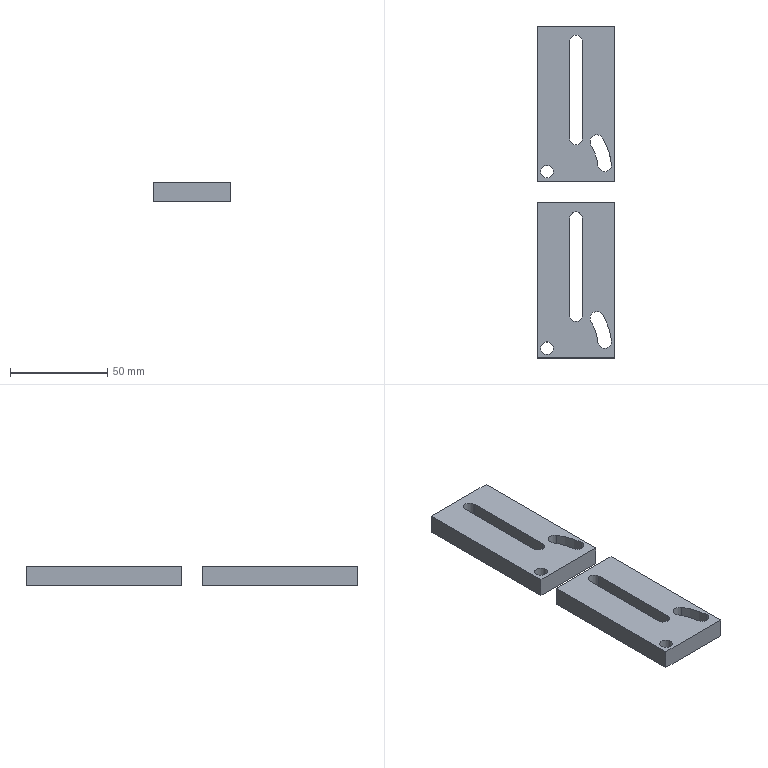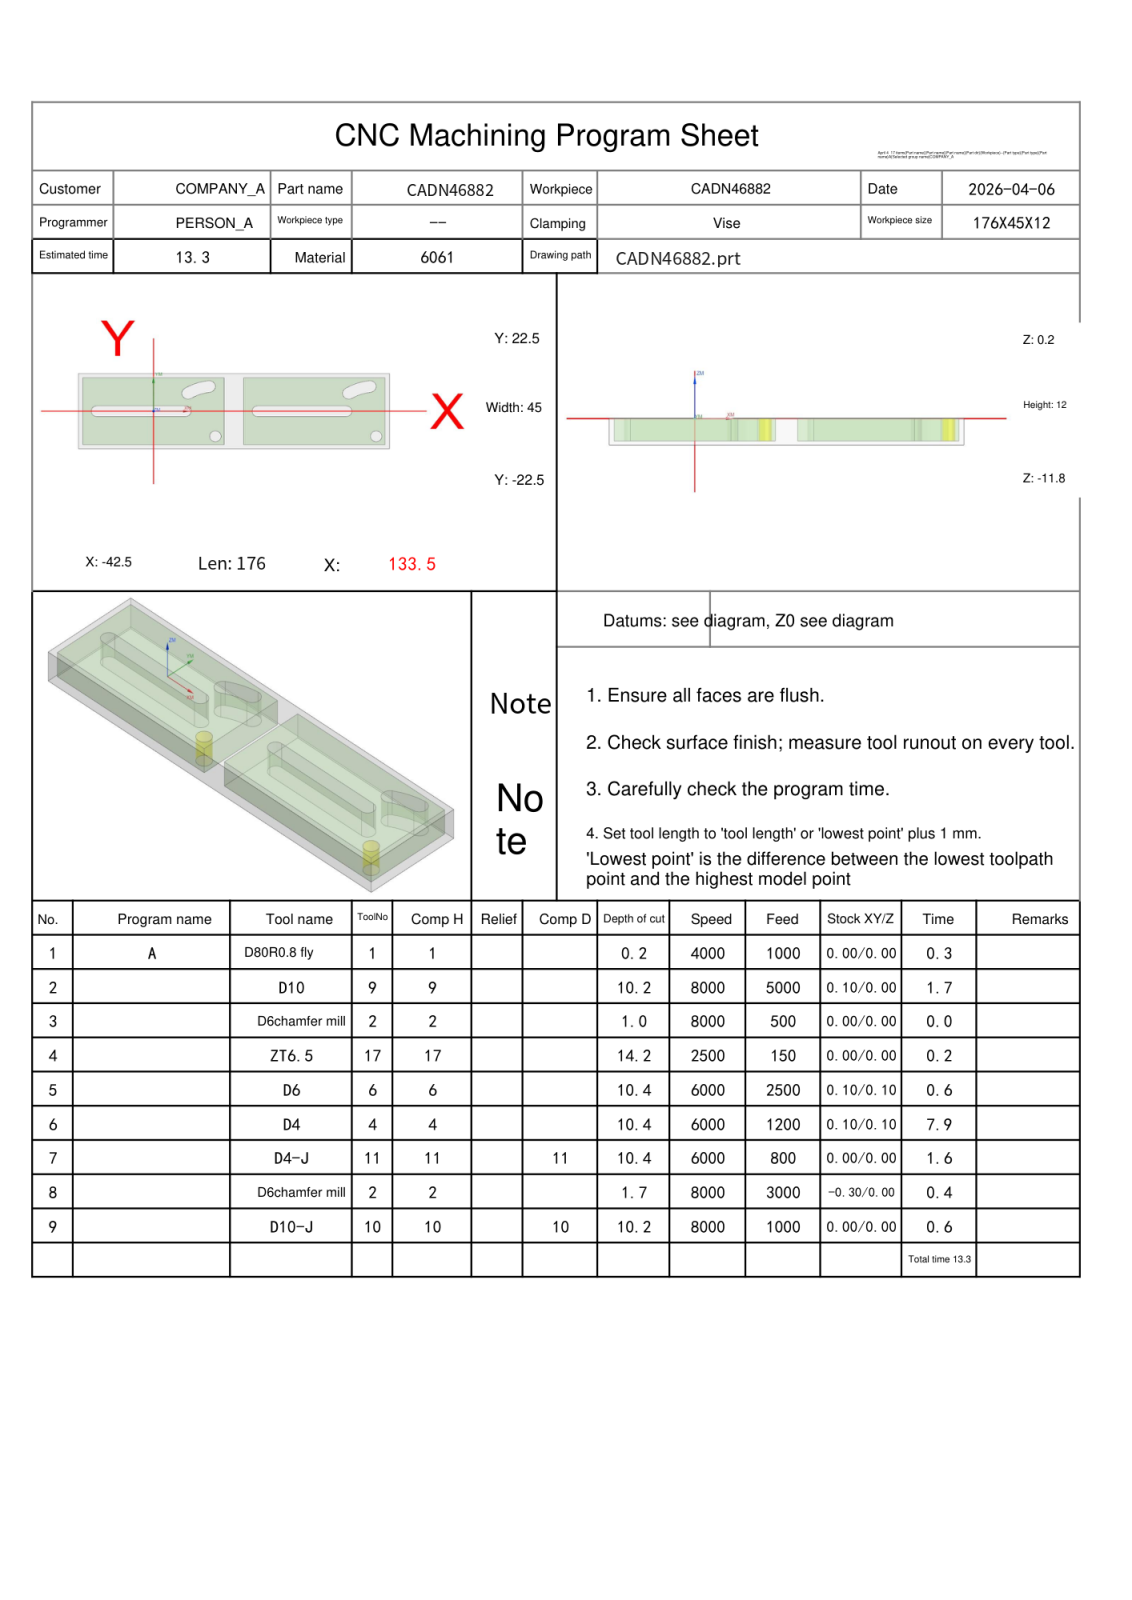NC program | NX | posted by the shop | part box 40 x 171 x 10 mm
Lines 1 to 1759 of 1806, first 1216 of 1757 lines:
%
O0001
(Machine time: 15.00 MIN)
(===Total Tool:8===)
(T1=D80R0.8 fly D=80.  R=0.8  D-  H01 Z=0.    )
(T9=D10     D=10.  R=0.   D-  H09 Z=-10.  )
(T2=D6chamfer mill   D=6.   R=0.   D-  H02 Z=-1.5  )
(T17=ZT6.5  D=6.5  DR_a=118 D-  H17 Z=-13.95)
(T6=D6      D=6.   R=0.   D-  H06 Z=-10.2 )
(T4=D4      D=4.   R=0.   D-  H04 Z=-10.2 )
(T11=D4-J   D=4.   R=0.   D11 H11 Z=-10.2 )
(T10=D10-J  D=10.  R=0.   D10 H10 Z=-10.  )
G80 G90 G17 G49 G40
G91 G28 Z0
M01
N1 T01 M06
(D80R0.8 fly  D=80. R=0.8 H=01 ce=0.00 di=0.00)
G00 G90 G54 X176. Y0.0 M03 S4000
G43 H01 Z20.
M08
Z2.
G01 Z0.0 F1000.
X171.
X-80.
X-85.
Z2.
G00 Z20.
G91 G28 Z0.0
M05
M09
G91 G28 Z0.0
M01
N2 T09 M06
(D10  D=10. R=0. H=09 ce=0.10 di=0.00)
G00 G90 G54 X91. Y-25.1 M03 S8000
G43 H09 Z20.
M08
Z.5
G01 X51. Z.39 F5000.
G02 X45.9 Y-20. Z.368 I0.0 J5.1
G01 Y20. Z.257
G02 X51. Y25.1 Z.235 I5.1 J0.0
G01 X131. Z.015
G02 X136.1 Y20. Z-.007 I0.0 J-5.1
G01 Y-20. Z-.118
G02 X131. Y-25.1 Z-.14 I-5.1 J0.0
G01 X51. Z-.36
G02 X45.9 Y-20. Z-.382 I0.0 J5.1
G01 Y20. Z-.493
G02 X51. Y25.1 Z-.515 I5.1 J0.0
G01 X131. Z-.735
G02 X136.1 Y20. Z-.757 I0.0 J-5.1
G01 Y-20. Z-.868
G02 X131. Y-25.1 Z-.89 I-5.1 J0.0
G01 X51. Z-1.11
G02 X45.9 Y-20. Z-1.132 I0.0 J5.1
G01 Y20. Z-1.243
G02 X51. Y25.1 Z-1.265 I5.1 J0.0
G01 X131. Z-1.485
G02 X136.1 Y20. Z-1.507 I0.0 J-5.1
G01 Y-20. Z-1.618
G02 X131. Y-25.1 Z-1.64 I-5.1 J0.0
G01 X51. Z-1.86
G02 X45.9 Y-20. Z-1.882 I0.0 J5.1
G01 Y20. Z-1.993
G02 X51. Y25.1 Z-2.015 I5.1 J0.0
G01 X131. Z-2.235
G02 X136.1 Y20. Z-2.257 I0.0 J-5.1
G01 Y-20. Z-2.368
G02 X131. Y-25.1 Z-2.39 I-5.1 J0.0
G01 X51. Z-2.61
G02 X45.9 Y-20. Z-2.632 I0.0 J5.1
G01 Y20. Z-2.743
G02 X51. Y25.1 Z-2.765 I5.1 J0.0
G01 X131. Z-2.985
G02 X136.1 Y20. Z-3.007 I0.0 J-5.1
G01 Y-20. Z-3.118
G02 X131. Y-25.1 Z-3.14 I-5.1 J0.0
G01 X51. Z-3.36
G02 X45.9 Y-20. Z-3.382 I0.0 J5.1
G01 Y20. Z-3.493
G02 X51. Y25.1 Z-3.515 I5.1 J0.0
G01 X131. Z-3.735
G02 X136.1 Y20. Z-3.757 I0.0 J-5.1
G01 Y-20. Z-3.868
G02 X131. Y-25.1 Z-3.89 I-5.1 J0.0
G01 X51. Z-4.11
G02 X45.9 Y-20. Z-4.132 I0.0 J5.1
G01 Y20. Z-4.243
G02 X51. Y25.1 Z-4.265 I5.1 J0.0
G01 X131. Z-4.485
G02 X136.1 Y20. Z-4.507 I0.0 J-5.1
G01 Y-20. Z-4.618
G02 X131. Y-25.1 Z-4.64 I-5.1 J0.0
G01 X51. Z-4.86
G02 X45.9 Y-20. Z-4.882 I0.0 J5.1
G01 Y20. Z-4.993
G02 X51. Y25.1 Z-5.015 I5.1 J0.0
G01 X131. Z-5.235
G02 X136.1 Y20. Z-5.257 I0.0 J-5.1
G01 Y-20. Z-5.368
G02 X131. Y-25.1 Z-5.39 I-5.1 J0.0
G01 X51. Z-5.61
G02 X45.9 Y-20. Z-5.632 I0.0 J5.1
G01 Y20. Z-5.743
G02 X51. Y25.1 Z-5.765 I5.1 J0.0
G01 X131. Z-5.985
G02 X136.1 Y20. Z-6.007 I0.0 J-5.1
G01 Y-20. Z-6.118
G02 X131. Y-25.1 Z-6.14 I-5.1 J0.0
G01 X51. Z-6.36
G02 X45.9 Y-20. Z-6.382 I0.0 J5.1
G01 Y20. Z-6.493
G02 X51. Y25.1 Z-6.515 I5.1 J0.0
G01 X131. Z-6.735
G02 X136.1 Y20. Z-6.757 I0.0 J-5.1
G01 Y-20. Z-6.868
G02 X131. Y-25.1 Z-6.89 I-5.1 J0.0
G01 X51. Z-7.11
G02 X45.9 Y-20. Z-7.132 I0.0 J5.1
G01 Y20. Z-7.243
G02 X51. Y25.1 Z-7.265 I5.1 J0.0
G01 X131. Z-7.485
G02 X136.1 Y20. Z-7.507 I0.0 J-5.1
G01 Y-20. Z-7.618
G02 X131. Y-25.1 Z-7.64 I-5.1 J0.0
G01 X51. Z-7.86
G02 X45.9 Y-20. Z-7.882 I0.0 J5.1
G01 Y20. Z-7.993
G02 X51. Y25.1 Z-8.015 I5.1 J0.0
G01 X131. Z-8.235
G02 X136.1 Y20. Z-8.257 I0.0 J-5.1
G01 Y-20. Z-8.368
G02 X131. Y-25.1 Z-8.39 I-5.1 J0.0
G01 X51. Z-8.61
G02 X45.9 Y-20. Z-8.632 I0.0 J5.1
G01 Y20. Z-8.743
G02 X51. Y25.1 Z-8.765 I5.1 J0.0
G01 X131. Z-8.985
G02 X136.1 Y20. Z-9.007 I0.0 J-5.1
G01 Y-20. Z-9.118
G02 X131. Y-25.1 Z-9.14 I-5.1 J0.0
G01 X51. Z-9.36
G02 X45.9 Y-20. Z-9.382 I0.0 J5.1
G01 Y20. Z-9.493
G02 X51. Y25.1 Z-9.515 I5.1 J0.0
G01 X131. Z-9.735
G02 X136.1 Y20. Z-9.757 I0.0 J-5.1
G01 Y-20. Z-9.868
G02 X131. Y-25.1 Z-9.89 I-5.1 J0.0
G01 X91. Z-10.
X51.
G02 X45.9 Y-20. I0.0 J5.1
G01 Y20.
G02 X51. Y25.1 I5.1 J0.0
G01 X131.
G02 X136.1 Y20. I0.0 J-5.1
G01 Y-20.
G02 X131. Y-25.1 I-5.1 J0.0
G01 X91.
X90.5
Z-9.
G00 Z20.
X0.0
Z.5
G01 X-40. Z.39
G02 X-45.1 Y-20. Z.368 I0.0 J5.1
G01 Y20. Z.257
G02 X-40. Y25.1 Z.235 I5.1 J0.0
G01 X40. Z.015
G02 X45.1 Y20. Z-.007 I0.0 J-5.1
G01 Y-20. Z-.118
G02 X40. Y-25.1 Z-.14 I-5.1 J0.0
G01 X-40. Z-.36
G02 X-45.1 Y-20. Z-.382 I0.0 J5.1
G01 Y20. Z-.493
G02 X-40. Y25.1 Z-.515 I5.1 J0.0
G01 X40. Z-.735
G02 X45.1 Y20. Z-.757 I0.0 J-5.1
G01 Y-20. Z-.868
G02 X40. Y-25.1 Z-.89 I-5.1 J0.0
G01 X-40. Z-1.11
G02 X-45.1 Y-20. Z-1.132 I0.0 J5.1
G01 Y20. Z-1.243
G02 X-40. Y25.1 Z-1.265 I5.1 J0.0
G01 X40. Z-1.485
G02 X45.1 Y20. Z-1.507 I0.0 J-5.1
G01 Y-20. Z-1.618
G02 X40. Y-25.1 Z-1.64 I-5.1 J0.0
G01 X-40. Z-1.86
G02 X-45.1 Y-20. Z-1.882 I0.0 J5.1
G01 Y20. Z-1.993
G02 X-40. Y25.1 Z-2.015 I5.1 J0.0
G01 X40. Z-2.235
G02 X45.1 Y20. Z-2.257 I0.0 J-5.1
G01 Y-20. Z-2.368
G02 X40. Y-25.1 Z-2.39 I-5.1 J0.0
G01 X-40. Z-2.61
G02 X-45.1 Y-20. Z-2.632 I0.0 J5.1
G01 Y20. Z-2.743
G02 X-40. Y25.1 Z-2.765 I5.1 J0.0
G01 X40. Z-2.985
G02 X45.1 Y20. Z-3.007 I0.0 J-5.1
G01 Y-20. Z-3.118
G02 X40. Y-25.1 Z-3.14 I-5.1 J0.0
G01 X-40. Z-3.36
G02 X-45.1 Y-20. Z-3.382 I0.0 J5.1
G01 Y20. Z-3.493
G02 X-40. Y25.1 Z-3.515 I5.1 J0.0
G01 X40. Z-3.735
G02 X45.1 Y20. Z-3.757 I0.0 J-5.1
G01 Y-20. Z-3.868
G02 X40. Y-25.1 Z-3.89 I-5.1 J0.0
G01 X-40. Z-4.11
G02 X-45.1 Y-20. Z-4.132 I0.0 J5.1
G01 Y20. Z-4.243
G02 X-40. Y25.1 Z-4.265 I5.1 J0.0
G01 X40. Z-4.485
G02 X45.1 Y20. Z-4.507 I0.0 J-5.1
G01 Y-20. Z-4.618
G02 X40. Y-25.1 Z-4.64 I-5.1 J0.0
G01 X-40. Z-4.86
G02 X-45.1 Y-20. Z-4.882 I0.0 J5.1
G01 Y20. Z-4.993
G02 X-40. Y25.1 Z-5.015 I5.1 J0.0
G01 X40. Z-5.235
G02 X45.1 Y20. Z-5.257 I0.0 J-5.1
G01 Y-20. Z-5.368
G02 X40. Y-25.1 Z-5.39 I-5.1 J0.0
G01 X-40. Z-5.61
G02 X-45.1 Y-20. Z-5.632 I0.0 J5.1
G01 Y20. Z-5.743
G02 X-40. Y25.1 Z-5.765 I5.1 J0.0
G01 X40. Z-5.985
G02 X45.1 Y20. Z-6.007 I0.0 J-5.1
G01 Y-20. Z-6.118
G02 X40. Y-25.1 Z-6.14 I-5.1 J0.0
G01 X-40. Z-6.36
G02 X-45.1 Y-20. Z-6.382 I0.0 J5.1
G01 Y20. Z-6.493
G02 X-40. Y25.1 Z-6.515 I5.1 J0.0
G01 X40. Z-6.735
G02 X45.1 Y20. Z-6.757 I0.0 J-5.1
G01 Y-20. Z-6.868
G02 X40. Y-25.1 Z-6.89 I-5.1 J0.0
G01 X-40. Z-7.11
G02 X-45.1 Y-20. Z-7.132 I0.0 J5.1
G01 Y20. Z-7.243
G02 X-40. Y25.1 Z-7.265 I5.1 J0.0
G01 X40. Z-7.485
G02 X45.1 Y20. Z-7.507 I0.0 J-5.1
G01 Y-20. Z-7.618
G02 X40. Y-25.1 Z-7.64 I-5.1 J0.0
G01 X-40. Z-7.86
G02 X-45.1 Y-20. Z-7.882 I0.0 J5.1
G01 Y20. Z-7.993
G02 X-40. Y25.1 Z-8.015 I5.1 J0.0
G01 X40. Z-8.235
G02 X45.1 Y20. Z-8.257 I0.0 J-5.1
G01 Y-20. Z-8.368
G02 X40. Y-25.1 Z-8.39 I-5.1 J0.0
G01 X-40. Z-8.61
G02 X-45.1 Y-20. Z-8.632 I0.0 J5.1
G01 Y20. Z-8.743
G02 X-40. Y25.1 Z-8.765 I5.1 J0.0
G01 X40. Z-8.985
G02 X45.1 Y20. Z-9.007 I0.0 J-5.1
G01 Y-20. Z-9.118
G02 X40. Y-25.1 Z-9.14 I-5.1 J0.0
G01 X-40. Z-9.36
G02 X-45.1 Y-20. Z-9.382 I0.0 J5.1
G01 Y20. Z-9.493
G02 X-40. Y25.1 Z-9.515 I5.1 J0.0
G01 X40. Z-9.735
G02 X45.1 Y20. Z-9.757 I0.0 J-5.1
G01 Y-20. Z-9.868
G02 X40. Y-25.1 Z-9.89 I-5.1 J0.0
G01 X0.0 Z-10.
X-40.
G02 X-45.1 Y-20. I0.0 J5.1
G01 Y20.
G02 X-40. Y25.1 I5.1 J0.0
G01 X40.
G02 X45.1 Y20. I0.0 J-5.1
G01 Y-20.
G02 X40. Y-25.1 I-5.1 J0.0
G01 X0.0
X-.5
Z-9.
G00 Z20.
G91 G28 Z0.0
M05
M09
G91 G28 Z0.0
M01
N3 T02 M06
(D6chamfer mill  D=6. R=0. H=02 ce=0.00 di=0.00)
G00 G90 G54 X35. Y-15. M03 S8000
G43 H02 Z20.
M08
G98 G81 X35. Y-15. Z-.8 R1. F500.
X126.
G80
G00 Z20.
G91 G28 Z0.0
M05
M09
G91 G28 Z0.0
M01
N4 T17 M06
(ZT6.5 D=6.5 DR_a=118 H=17)
G00 G90 G54 X35. Y-15. M03 S2500
G43 H17 Z20.
M08
G98 G83 X35. Y-15. Z-13.953 R1. F150. Q3.
X126.
G80
G00 Z20.
G91 G28 Z0.0
M05
M09
G91 G28 Z0.0
M01
N5 T06 M06
(D6  D=6. R=0. H=06 ce=0.10 di=0.10)
G00 G90 G54 X116.174 Y13.768 M03 S6000
G43 H06 Z20.
M08
Z.5
G03 X110.335 Y11.053 Z.409 I9.826 J-28.768 F2500.
G01 X110.281 Y11.028 Z.408
X110.246 Y10.98 Z.407
G03 X110.199 Y10.504 Z.4 I.296 J-.269
X110.748 Y10.368 Z.391 I.343 J.206
G02 X122.547 Y14.398 Z.213 I15.252 J-25.368
G03 X122.897 Y14.842 Z.204 I-.047 J.397
X122.453 Y15.192 Z.195 I-.397 J-.047
X116.174 Y13.768 Z.104 I3.547 J-30.192
X110.335 Y11.053 Z.012 I9.826 J-28.768
G01 X110.281 Y11.028
X110.246 Y10.98 Z.011
G03 X110.199 Y10.504 Z.003 I.296 J-.269
X110.748 Y10.368 Z-.005 I.343 J.206
G02 X122.547 Y14.398 Z-.183 I15.252 J-25.368
G03 X122.897 Y14.842 Z-.192 I-.047 J.397
X122.453 Y15.192 Z-.201 I-.397 J-.047
X116.174 Y13.768 Z-.293 I3.547 J-30.192
X110.335 Y11.053 Z-.384 I9.826 J-28.768
G01 X110.281 Y11.028 Z-.385
X110.246 Y10.98 Z-.386
G03 X110.199 Y10.504 Z-.393 I.296 J-.269
X110.748 Y10.368 Z-.402 I.343 J.206
G02 X122.547 Y14.398 Z-.58 I15.252 J-25.368
G03 X122.897 Y14.842 Z-.589 I-.047 J.397
X122.453 Y15.192 Z-.598 I-.397 J-.047
X116.174 Y13.768 Z-.689 I3.547 J-30.192
X110.335 Y11.053 Z-.78 I9.826 J-28.768
G01 X110.281 Y11.028 Z-.781
X110.246 Y10.98 Z-.782
G03 X110.199 Y10.504 Z-.789 I.296 J-.269
X110.748 Y10.368 Z-.798 I.343 J.206
G02 X122.547 Y14.398 Z-.976 I15.252 J-25.368
G03 X122.897 Y14.842 Z-.985 I-.047 J.397
X122.453 Y15.192 Z-.994 I-.397 J-.047
X116.174 Y13.768 Z-1.085 I3.547 J-30.192
X110.335 Y11.053 Z-1.177 I9.826 J-28.768
G01 X110.281 Y11.028
X110.246 Y10.98 Z-1.178
G03 X110.199 Y10.504 Z-1.185 I.296 J-.269
X110.748 Y10.368 Z-1.194 I.343 J.206
G02 X122.547 Y14.398 Z-1.372 I15.252 J-25.368
G03 X122.897 Y14.842 Z-1.381 I-.047 J.397
X122.453 Y15.192 Z-1.39 I-.397 J-.047
X116.174 Y13.768 Z-1.481 I3.547 J-30.192
X110.335 Y11.053 Z-1.573 I9.826 J-28.768
G01 X110.281 Y11.028 Z-1.574
X110.246 Y10.98 Z-1.575
G03 X110.199 Y10.504 Z-1.582 I.296 J-.269
X110.748 Y10.368 Z-1.591 I.343 J.206
G02 X122.547 Y14.398 Z-1.769 I15.252 J-25.368
G03 X122.897 Y14.842 Z-1.778 I-.047 J.397
X122.453 Y15.192 Z-1.786 I-.397 J-.047
X116.174 Y13.768 Z-1.878 I3.547 J-30.192
X110.335 Y11.053 Z-1.969 I9.826 J-28.768
G01 X110.281 Y11.028 Z-1.97
X110.246 Y10.98 Z-1.971
G03 X110.199 Y10.504 Z-1.978 I.296 J-.269
X110.748 Y10.368 Z-1.987 I.343 J.206
G02 X122.547 Y14.398 Z-2.165 I15.252 J-25.368
G03 X122.897 Y14.842 Z-2.174 I-.047 J.397
X122.453 Y15.192 Z-2.183 I-.397 J-.047
X116.174 Y13.768 Z-2.274 I3.547 J-30.192
X110.335 Y11.053 Z-2.365 I9.826 J-28.768
G01 X110.281 Y11.028 Z-2.366
X110.246 Y10.98 Z-2.367
G03 X110.199 Y10.504 Z-2.374 I.296 J-.269
X110.748 Y10.368 Z-2.383 I.343 J.206
G02 X122.547 Y14.398 Z-2.561 I15.252 J-25.368
G03 X122.897 Y14.842 Z-2.57 I-.047 J.397
X122.453 Y15.192 Z-2.579 I-.397 J-.047
X116.174 Y13.768 Z-2.67 I3.547 J-30.192
X110.335 Y11.053 Z-2.762 I9.826 J-28.768
G01 X110.281 Y11.028 Z-2.763
X110.246 Y10.98
G03 X110.199 Y10.504 Z-2.771 I.296 J-.269
X110.748 Y10.368 Z-2.78 I.343 J.206
G02 X122.547 Y14.398 Z-2.957 I15.252 J-25.368
G03 X122.897 Y14.842 Z-2.966 I-.047 J.397
X122.453 Y15.192 Z-2.975 I-.397 J-.047
X116.174 Y13.768 Z-3.067 I3.547 J-30.192
X110.335 Y11.053 Z-3.158 I9.826 J-28.768
G01 X110.281 Y11.028 Z-3.159
X110.246 Y10.98 Z-3.16
G03 X110.199 Y10.504 Z-3.167 I.296 J-.269
X110.748 Y10.368 Z-3.176 I.343 J.206
G02 X122.547 Y14.398 Z-3.354 I15.252 J-25.368
G03 X122.897 Y14.842 Z-3.363 I-.047 J.397
X122.453 Y15.192 Z-3.372 I-.397 J-.047
X116.174 Y13.768 Z-3.463 I3.547 J-30.192
X110.335 Y11.053 Z-3.554 I9.826 J-28.768
G01 X110.281 Y11.028 Z-3.555
X110.246 Y10.98 Z-3.556
G03 X110.199 Y10.504 Z-3.563 I.296 J-.269
X110.748 Y10.368 Z-3.572 I.343 J.206
G02 X122.547 Y14.398 Z-3.75 I15.252 J-25.368
G03 X122.897 Y14.842 Z-3.759 I-.047 J.397
X122.453 Y15.192 Z-3.768 I-.397 J-.047
X116.174 Y13.768 Z-3.859 I3.547 J-30.192
X110.335 Y11.053 Z-3.951 I9.826 J-28.768
G01 X110.281 Y11.028
X110.246 Y10.98 Z-3.952
G03 X110.199 Y10.504 Z-3.96 I.296 J-.269
X110.748 Y10.368 Z-3.968 I.343 J.206
G02 X122.547 Y14.398 Z-4.146 I15.252 J-25.368
G03 X122.897 Y14.842 Z-4.155 I-.047 J.397
X122.453 Y15.192 Z-4.164 I-.397 J-.047
X116.174 Y13.768 Z-4.256 I3.547 J-30.192
X110.335 Y11.053 Z-4.347 I9.826 J-28.768
G01 X110.281 Y11.028 Z-4.348
X110.246 Y10.98 Z-4.349
G03 X110.199 Y10.504 Z-4.356 I.296 J-.269
X110.748 Y10.368 Z-4.365 I.343 J.206
G02 X122.547 Y14.398 Z-4.543 I15.252 J-25.368
G03 X122.897 Y14.842 Z-4.552 I-.047 J.397
X122.453 Y15.192 Z-4.56 I-.397 J-.047
X116.174 Y13.768 Z-4.652 I3.547 J-30.192
X110.335 Y11.053 Z-4.743 I9.826 J-28.768
G01 X110.281 Y11.028 Z-4.744
X110.246 Y10.98 Z-4.745
G03 X110.199 Y10.504 Z-4.752 I.296 J-.269
X110.748 Y10.368 Z-4.761 I.343 J.206
G02 X122.547 Y14.398 Z-4.939 I15.252 J-25.368
G03 X122.897 Y14.842 Z-4.948 I-.047 J.397
X122.453 Y15.192 Z-4.957 I-.397 J-.047
X116.174 Y13.768 Z-5.048 I3.547 J-30.192
X110.335 Y11.053 Z-5.14 I9.826 J-28.768
G01 X110.281 Y11.028
X110.246 Y10.98 Z-5.141
G03 X110.199 Y10.504 Z-5.148 I.296 J-.269
X110.748 Y10.368 Z-5.157 I.343 J.206
G02 X122.547 Y14.398 Z-5.335 I15.252 J-25.368
G03 X122.897 Y14.842 Z-5.344 I-.047 J.397
X122.453 Y15.192 Z-5.353 I-.397 J-.047
X116.174 Y13.768 Z-5.444 I3.547 J-30.192
X110.335 Y11.053 Z-5.536 I9.826 J-28.768
G01 X110.281 Y11.028 Z-5.537
X110.246 Y10.98
G03 X110.199 Y10.504 Z-5.545 I.296 J-.269
X110.748 Y10.368 Z-5.554 I.343 J.206
G02 X122.547 Y14.398 Z-5.732 I15.252 J-25.368
G03 X122.897 Y14.842 Z-5.74 I-.047 J.397
X122.453 Y15.192 Z-5.749 I-.397 J-.047
X116.174 Y13.768 Z-5.841 I3.547 J-30.192
X110.335 Y11.053 Z-5.932 I9.826 J-28.768
G01 X110.281 Y11.028 Z-5.933
X110.246 Y10.98 Z-5.934
G03 X110.199 Y10.504 Z-5.941 I.296 J-.269
X110.748 Y10.368 Z-5.95 I.343 J.206
G02 X122.547 Y14.398 Z-6.128 I15.252 J-25.368
G03 X122.897 Y14.842 Z-6.137 I-.047 J.397
X122.453 Y15.192 Z-6.146 I-.397 J-.047
X116.174 Y13.768 Z-6.237 I3.547 J-30.192
X110.335 Y11.053 Z-6.328 I9.826 J-28.768
G01 X110.281 Y11.028 Z-6.329
X110.246 Y10.98 Z-6.33
G03 X110.199 Y10.504 Z-6.337 I.296 J-.269
X110.748 Y10.368 Z-6.346 I.343 J.206
G02 X122.547 Y14.398 Z-6.524 I15.252 J-25.368
G03 X122.897 Y14.842 Z-6.533 I-.047 J.397
X122.453 Y15.192 Z-6.542 I-.397 J-.047
X116.174 Y13.768 Z-6.633 I3.547 J-30.192
X110.335 Y11.053 Z-6.725 I9.826 J-28.768
G01 X110.281 Y11.028 Z-6.726
X110.246 Y10.98
G03 X110.199 Y10.504 Z-6.734 I.296 J-.269
X110.748 Y10.368 Z-6.743 I.343 J.206
G02 X122.547 Y14.398 Z-6.92 I15.252 J-25.368
G03 X122.897 Y14.842 Z-6.929 I-.047 J.397
X122.453 Y15.192 Z-6.938 I-.397 J-.047
X116.174 Y13.768 Z-7.03 I3.547 J-30.192
X110.335 Y11.053 Z-7.121 I9.826 J-28.768
G01 X110.281 Y11.028 Z-7.122
X110.246 Y10.98 Z-7.123
G03 X110.199 Y10.504 Z-7.13 I.296 J-.269
X110.748 Y10.368 Z-7.139 I.343 J.206
G02 X122.547 Y14.398 Z-7.317 I15.252 J-25.368
G03 X122.897 Y14.842 Z-7.326 I-.047 J.397
X122.453 Y15.192 Z-7.335 I-.397 J-.047
X116.174 Y13.768 Z-7.426 I3.547 J-30.192
X110.335 Y11.053 Z-7.517 I9.826 J-28.768
G01 X110.281 Y11.028 Z-7.518
X110.246 Y10.98 Z-7.519
G03 X110.199 Y10.504 Z-7.526 I.296 J-.269
X110.748 Y10.368 Z-7.535 I.343 J.206
G02 X122.547 Y14.398 Z-7.713 I15.252 J-25.368
G03 X122.897 Y14.842 Z-7.722 I-.047 J.397
X122.453 Y15.192 Z-7.731 I-.397 J-.047
X116.174 Y13.768 Z-7.822 I3.547 J-30.192
X110.335 Y11.053 Z-7.914 I9.826 J-28.768
G01 X110.281 Y11.028
X110.246 Y10.98 Z-7.915
G03 X110.199 Y10.504 Z-7.922 I.296 J-.269
X110.748 Y10.368 Z-7.931 I.343 J.206
G02 X122.547 Y14.398 Z-8.109 I15.252 J-25.368
G03 X122.897 Y14.842 Z-8.118 I-.047 J.397
X122.453 Y15.192 Z-8.127 I-.397 J-.047
X116.174 Y13.768 Z-8.219 I3.547 J-30.192
X110.335 Y11.053 Z-8.31 I9.826 J-28.768
G01 X110.281 Y11.028 Z-8.311
X110.246 Y10.98 Z-8.312
G03 X110.199 Y10.504 Z-8.319 I.296 J-.269
X110.748 Y10.368 Z-8.328 I.343 J.206
G02 X122.547 Y14.398 Z-8.506 I15.252 J-25.368
G03 X122.897 Y14.842 Z-8.515 I-.047 J.397
X122.453 Y15.192 Z-8.523 I-.397 J-.047
X116.174 Y13.768 Z-8.615 I3.547 J-30.192
X110.335 Y11.053 Z-8.706 I9.826 J-28.768
G01 X110.281 Y11.028 Z-8.707
X110.246 Y10.98 Z-8.708
G03 X110.199 Y10.504 Z-8.715 I.296 J-.269
X110.748 Y10.368 Z-8.724 I.343 J.206
G02 X122.547 Y14.398 Z-8.902 I15.252 J-25.368
G03 X122.897 Y14.842 Z-8.911 I-.047 J.397
X122.453 Y15.192 Z-8.92 I-.397 J-.047
X116.174 Y13.768 Z-9.011 I3.547 J-30.192
X110.335 Y11.053 Z-9.102 I9.826 J-28.768
G01 X110.281 Y11.028 Z-9.103
X110.246 Y10.98 Z-9.104
G03 X110.199 Y10.504 Z-9.111 I.296 J-.269
X110.748 Y10.368 Z-9.12 I.343 J.206
G02 X122.547 Y14.398 Z-9.298 I15.252 J-25.368
G03 X122.897 Y14.842 Z-9.307 I-.047 J.397
X122.453 Y15.192 Z-9.316 I-.397 J-.047
X116.174 Y13.768 Z-9.407 I3.547 J-30.192
X110.335 Y11.053 Z-9.499 I9.826 J-28.768
G01 X110.281 Y11.028 Z-9.5
X110.246 Y10.98
G03 X110.199 Y10.504 Z-9.508 I.296 J-.269
X110.748 Y10.368 Z-9.517 I.343 J.206
G02 X122.547 Y14.398 Z-9.695 I15.252 J-25.368
G03 X122.897 Y14.842 Z-9.703 I-.047 J.397
X122.453 Y15.192 Z-9.712 I-.397 J-.047
X116.174 Y13.768 Z-9.804 I3.547 J-30.192
X110.335 Y11.053 Z-9.895 I9.826 J-28.768
G01 X110.281 Y11.028 Z-9.896
X110.246 Y10.98 Z-9.897
G03 X110.199 Y10.504 Z-9.904 I.296 J-.269
X110.748 Y10.368 Z-9.913 I.343 J.206
G02 X122.547 Y14.398 Z-10.091 I15.252 J-25.368
G03 X122.897 Y14.842 Z-10.1 I-.047 J.397
X122.453 Y15.192 Z-10.109 I-.397 J-.047
X116.174 Y13.768 Z-10.2 I3.547 J-30.192
X110.335 Y11.053 I9.826 J-28.768
X110.141 Y10.711 I.206 J-.343
X110.541 Y10.311 I.4 J0.0
X110.748 Y10.368 I0.0 J.4
G02 X122.547 Y14.398 I15.252 J-25.368
G03 X122.9 Y14.795 I-.047 J.397
X122.5 Y15.195 I-.4 J0.0
G01 X122.453 Y15.192
G03 X116.174 Y13.768 I3.547 J-30.192
X115.702 Y13.603 I9.826 J-28.768
G01 Z-9.2
G00 Z20.
X31.894 Y14.863
Z.5
G01 X31.89 Y14.884
G03 X31.698 Y15.143 Z.495 I-.39 J-.089
X31.453 Y15.192 Z.491 I-.198 J-.348
X19.335 Y11.053 Z.309 I3.547 J-30.192
X19.199 Y10.504 Z.3 I.206 J-.343
X19.748 Y10.368 Z.291 I.343 J.206
G02 X31.547 Y14.398 Z.113 I15.252 J-25.368
G03 X31.897 Y14.842 Z.104 I-.047 J.397
G01 X31.894 Y14.863
X31.89 Y14.884 Z.103
G03 X31.698 Y15.143 Z.099 I-.39 J-.089
X31.453 Y15.192 Z.095 I-.198 J-.348
X19.335 Y11.053 Z-.088 I3.547 J-30.192
X19.199 Y10.504 Z-.097 I.206 J-.343
X19.748 Y10.368 Z-.105 I.343 J.206
G02 X31.547 Y14.398 Z-.283 I15.252 J-25.368
G03 X31.897 Y14.842 Z-.292 I-.047 J.397
G01 X31.894 Y14.863 Z-.293
X31.89 Y14.884
G03 X31.698 Y15.143 Z-.298 I-.39 J-.089
X31.453 Y15.192 Z-.301 I-.198 J-.348
X19.335 Y11.053 Z-.484 I3.547 J-30.192
X19.199 Y10.504 Z-.493 I.206 J-.343
X19.748 Y10.368 Z-.502 I.343 J.206
G02 X31.547 Y14.398 Z-.68 I15.252 J-25.368
G03 X31.897 Y14.842 Z-.689 I-.047 J.397
G01 X31.894 Y14.863
X31.89 Y14.884
G03 X31.698 Y15.143 Z-.694 I-.39 J-.089
X31.453 Y15.192 Z-.697 I-.198 J-.348
X19.335 Y11.053 Z-.88 I3.547 J-30.192
X19.199 Y10.504 Z-.889 I.206 J-.343
X19.748 Y10.368 Z-.898 I.343 J.206
G02 X31.547 Y14.398 Z-1.076 I15.252 J-25.368
G03 X31.897 Y14.842 Z-1.085 I-.047 J.397
G01 X31.894 Y14.863
X31.89 Y14.884
G03 X31.698 Y15.143 Z-1.09 I-.39 J-.089
X31.453 Y15.192 Z-1.094 I-.198 J-.348
X19.335 Y11.053 Z-1.277 I3.547 J-30.192
X19.199 Y10.504 Z-1.285 I.206 J-.343
X19.748 Y10.368 Z-1.294 I.343 J.206
G02 X31.547 Y14.398 Z-1.472 I15.252 J-25.368
G03 X31.897 Y14.842 Z-1.481 I-.047 J.397
G01 X31.894 Y14.863
X31.89 Y14.884 Z-1.482
G03 X31.698 Y15.143 Z-1.486 I-.39 J-.089
X31.453 Y15.192 Z-1.49 I-.198 J-.348
X19.335 Y11.053 Z-1.673 I3.547 J-30.192
X19.199 Y10.504 Z-1.682 I.206 J-.343
X19.748 Y10.368 Z-1.691 I.343 J.206
G02 X31.547 Y14.398 Z-1.869 I15.252 J-25.368
G03 X31.897 Y14.842 Z-1.877 I-.047 J.397
G01 X31.894 Y14.863 Z-1.878
X31.89 Y14.884
G03 X31.698 Y15.143 Z-1.883 I-.39 J-.089
X31.453 Y15.192 Z-1.886 I-.198 J-.348
X19.335 Y11.053 Z-2.069 I3.547 J-30.192
X19.199 Y10.504 Z-2.078 I.206 J-.343
X19.748 Y10.368 Z-2.087 I.343 J.206
G02 X31.547 Y14.398 Z-2.265 I15.252 J-25.368
G03 X31.897 Y14.842 Z-2.274 I-.047 J.397
G01 X31.894 Y14.863
X31.89 Y14.884
G03 X31.698 Y15.143 Z-2.279 I-.39 J-.089
X31.453 Y15.192 Z-2.283 I-.198 J-.348
X19.335 Y11.053 Z-2.465 I3.547 J-30.192
X19.199 Y10.504 Z-2.474 I.206 J-.343
X19.748 Y10.368 Z-2.483 I.343 J.206
G02 X31.547 Y14.398 Z-2.661 I15.252 J-25.368
G03 X31.897 Y14.842 Z-2.67 I-.047 J.397
G01 X31.894 Y14.863
X31.89 Y14.884 Z-2.671
G03 X31.698 Y15.143 Z-2.675 I-.39 J-.089
X31.453 Y15.192 Z-2.679 I-.198 J-.348
X19.335 Y11.053 Z-2.862 I3.547 J-30.192
X19.199 Y10.504 Z-2.871 I.206 J-.343
X19.748 Y10.368 Z-2.88 I.343 J.206
G02 X31.547 Y14.398 Z-3.057 I15.252 J-25.368
G03 X31.897 Y14.842 Z-3.066 I-.047 J.397
G01 X31.894 Y14.863 Z-3.067
X31.89 Y14.884
G03 X31.698 Y15.143 Z-3.072 I-.39 J-.089
X31.453 Y15.192 Z-3.075 I-.198 J-.348
X19.335 Y11.053 Z-3.258 I3.547 J-30.192
X19.199 Y10.504 Z-3.267 I.206 J-.343
X19.748 Y10.368 Z-3.276 I.343 J.206
G02 X31.547 Y14.398 Z-3.454 I15.252 J-25.368
G03 X31.897 Y14.842 Z-3.463 I-.047 J.397
G01 X31.894 Y14.863
X31.89 Y14.884
G03 X31.698 Y15.143 Z-3.468 I-.39 J-.089
X31.453 Y15.192 Z-3.472 I-.198 J-.348
X19.335 Y11.053 Z-3.654 I3.547 J-30.192
X19.199 Y10.504 Z-3.663 I.206 J-.343
X19.748 Y10.368 Z-3.672 I.343 J.206
G02 X31.547 Y14.398 Z-3.85 I15.252 J-25.368
G03 X31.897 Y14.842 Z-3.859 I-.047 J.397
G01 X31.894 Y14.863
X31.89 Y14.884 Z-3.86
G03 X31.698 Y15.143 Z-3.864 I-.39 J-.089
X31.453 Y15.192 Z-3.868 I-.198 J-.348
X19.335 Y11.053 Z-4.051 I3.547 J-30.192
X19.199 Y10.504 Z-4.06 I.206 J-.343
X19.748 Y10.368 Z-4.068 I.343 J.206
G02 X31.547 Y14.398 Z-4.246 I15.252 J-25.368
G03 X31.897 Y14.842 Z-4.255 I-.047 J.397
G01 X31.894 Y14.863 Z-4.256
X31.89 Y14.884
G03 X31.698 Y15.143 Z-4.261 I-.39 J-.089
X31.453 Y15.192 Z-4.264 I-.198 J-.348
X19.335 Y11.053 Z-4.447 I3.547 J-30.192
X19.199 Y10.504 Z-4.456 I.206 J-.343
X19.748 Y10.368 Z-4.465 I.343 J.206
G02 X31.547 Y14.398 Z-4.643 I15.252 J-25.368
G03 X31.897 Y14.842 Z-4.652 I-.047 J.397
G01 X31.894 Y14.863
X31.89 Y14.884
G03 X31.698 Y15.143 Z-4.657 I-.39 J-.089
X31.453 Y15.192 Z-4.66 I-.198 J-.348
X19.335 Y11.053 Z-4.843 I3.547 J-30.192
X19.199 Y10.504 Z-4.852 I.206 J-.343
X19.748 Y10.368 Z-4.861 I.343 J.206
G02 X31.547 Y14.398 Z-5.039 I15.252 J-25.368
G03 X31.897 Y14.842 Z-5.048 I-.047 J.397
G01 X31.894 Y14.863
X31.89 Y14.884
G03 X31.698 Y15.143 Z-5.053 I-.39 J-.089
X31.453 Y15.192 Z-5.057 I-.198 J-.348
X19.335 Y11.053 Z-5.239 I3.547 J-30.192
X19.199 Y10.504 Z-5.248 I.206 J-.343
X19.748 Y10.368 Z-5.257 I.343 J.206
G02 X31.547 Y14.398 Z-5.435 I15.252 J-25.368
G03 X31.897 Y14.842 Z-5.444 I-.047 J.397
G01 X31.894 Y14.863
X31.89 Y14.884 Z-5.445
G03 X31.698 Y15.143 Z-5.449 I-.39 J-.089
X31.453 Y15.192 Z-5.453 I-.198 J-.348
X19.335 Y11.053 Z-5.636 I3.547 J-30.192
X19.199 Y10.504 Z-5.645 I.206 J-.343
X19.748 Y10.368 Z-5.654 I.343 J.206
G02 X31.547 Y14.398 Z-5.832 I15.252 J-25.368
G03 X31.897 Y14.842 Z-5.84 I-.047 J.397
G01 X31.894 Y14.863 Z-5.841
X31.89 Y14.884
G03 X31.698 Y15.143 Z-5.846 I-.39 J-.089
X31.453 Y15.192 Z-5.849 I-.198 J-.348
X19.335 Y11.053 Z-6.032 I3.547 J-30.192
X19.199 Y10.504 Z-6.041 I.206 J-.343
X19.748 Y10.368 Z-6.05 I.343 J.206
G02 X31.547 Y14.398 Z-6.228 I15.252 J-25.368
G03 X31.897 Y14.842 Z-6.237 I-.047 J.397
G01 X31.894 Y14.863
X31.89 Y14.884
G03 X31.698 Y15.143 Z-6.242 I-.39 J-.089
X31.453 Y15.192 Z-6.246 I-.198 J-.348
X19.335 Y11.053 Z-6.428 I3.547 J-30.192
X19.199 Y10.504 Z-6.437 I.206 J-.343
X19.748 Y10.368 Z-6.446 I.343 J.206
G02 X31.547 Y14.398 Z-6.624 I15.252 J-25.368
G03 X31.897 Y14.842 Z-6.633 I-.047 J.397
G01 X31.894 Y14.863
X31.89 Y14.884 Z-6.634
G03 X31.698 Y15.143 Z-6.638 I-.39 J-.089
X31.453 Y15.192 Z-6.642 I-.198 J-.348
X19.335 Y11.053 Z-6.825 I3.547 J-30.192
X19.199 Y10.504 Z-6.834 I.206 J-.343
X19.748 Y10.368 Z-6.842 I.343 J.206
G02 X31.547 Y14.398 Z-7.02 I15.252 J-25.368
G03 X31.897 Y14.842 Z-7.029 I-.047 J.397
G01 X31.894 Y14.863 Z-7.03
X31.89 Y14.884
G03 X31.698 Y15.143 Z-7.035 I-.39 J-.089
X31.453 Y15.192 Z-7.038 I-.198 J-.348
X19.335 Y11.053 Z-7.221 I3.547 J-30.192
X19.199 Y10.504 Z-7.23 I.206 J-.343
X19.748 Y10.368 Z-7.239 I.343 J.206
G02 X31.547 Y14.398 Z-7.417 I15.252 J-25.368
G03 X31.897 Y14.842 Z-7.426 I-.047 J.397
G01 X31.894 Y14.863
X31.89 Y14.884
G03 X31.698 Y15.143 Z-7.431 I-.39 J-.089
X31.453 Y15.192 Z-7.435 I-.198 J-.348
X19.335 Y11.053 Z-7.617 I3.547 J-30.192
X19.199 Y10.504 Z-7.626 I.206 J-.343
X19.748 Y10.368 Z-7.635 I.343 J.206
G02 X31.547 Y14.398 Z-7.813 I15.252 J-25.368
G03 X31.897 Y14.842 Z-7.822 I-.047 J.397
G01 X31.894 Y14.863
X31.89 Y14.884 Z-7.823
G03 X31.698 Y15.143 Z-7.827 I-.39 J-.089
X31.453 Y15.192 Z-7.831 I-.198 J-.348
X19.335 Y11.053 Z-8.014 I3.547 J-30.192
X19.199 Y10.504 Z-8.022 I.206 J-.343
X19.748 Y10.368 Z-8.031 I.343 J.206
G02 X31.547 Y14.398 Z-8.209 I15.252 J-25.368
G03 X31.897 Y14.842 Z-8.218 I-.047 J.397
G01 X31.894 Y14.863 Z-8.219
X31.89 Y14.884
G03 X31.698 Y15.143 Z-8.224 I-.39 J-.089
X31.453 Y15.192 Z-8.227 I-.198 J-.348
X19.335 Y11.053 Z-8.41 I3.547 J-30.192
X19.199 Y10.504 Z-8.419 I.206 J-.343
X19.748 Y10.368 Z-8.428 I.343 J.206
G02 X31.547 Y14.398 Z-8.606 I15.252 J-25.368
G03 X31.897 Y14.842 Z-8.615 I-.047 J.397
G01 X31.894 Y14.863
X31.89 Y14.884
G03 X31.698 Y15.143 Z-8.62 I-.39 J-.089
X31.453 Y15.192 Z-8.623 I-.198 J-.348
X19.335 Y11.053 Z-8.806 I3.547 J-30.192
X19.199 Y10.504 Z-8.815 I.206 J-.343
X19.748 Y10.368 Z-8.824 I.343 J.206
G02 X31.547 Y14.398 Z-9.002 I15.252 J-25.368
G03 X31.897 Y14.842 Z-9.011 I-.047 J.397
G01 X31.894 Y14.863
X31.89 Y14.884
G03 X31.698 Y15.143 Z-9.016 I-.39 J-.089
X31.453 Y15.192 Z-9.02 I-.198 J-.348
X19.335 Y11.053 Z-9.202 I3.547 J-30.192
X19.199 Y10.504 Z-9.211 I.206 J-.343
X19.748 Y10.368 Z-9.22 I.343 J.206
G02 X31.547 Y14.398 Z-9.398 I15.252 J-25.368
G03 X31.897 Y14.842 Z-9.407 I-.047 J.397
G01 X31.894 Y14.863
X31.89 Y14.884 Z-9.408
G03 X31.698 Y15.143 Z-9.412 I-.39 J-.089
X31.453 Y15.192 Z-9.416 I-.198 J-.348
X19.335 Y11.053 Z-9.599 I3.547 J-30.192
X19.199 Y10.504 Z-9.608 I.206 J-.343
X19.748 Y10.368 Z-9.617 I.343 J.206
G02 X31.547 Y14.398 Z-9.794 I15.252 J-25.368
G03 X31.897 Y14.842 Z-9.803 I-.047 J.397
G01 X31.894 Y14.863 Z-9.804
X31.89 Y14.884
G03 X31.698 Y15.143 Z-9.809 I-.39 J-.089
X31.453 Y15.192 Z-9.812 I-.198 J-.348
X19.335 Y11.053 Z-9.995 I3.547 J-30.192
X19.199 Y10.504 Z-10.004 I.206 J-.343
X19.748 Y10.368 Z-10.013 I.343 J.206
G02 X31.547 Y14.398 Z-10.191 I15.252 J-25.368
G03 X31.897 Y14.842 Z-10.2 I-.047 J.397
G01 X31.894 Y14.863
X31.89 Y14.884
G03 X31.5 Y15.195 I-.39 J-.089
G01 X31.453 Y15.192
G03 X19.335 Y11.053 I3.547 J-30.192
X19.141 Y10.711 I.206 J-.343
X19.541 Y10.311 I.4 J0.0
X19.748 Y10.368 I0.0 J.4
G02 X31.547 Y14.398 I15.252 J-25.368
G03 X31.9 Y14.795 I-.047 J.397
G01 X31.894 Y14.863
X31.89 Y14.884
G03 X31.56 Y15.191 I-.39 J-.089
G01 Z-9.2
G00 Z20.
G91 G28 Z0.0
M05
M09
G91 G28 Z0.0
M01
N6 T04 M06
(D4  D=4. R=0. H=04 ce=0.10 di=0.10)
G00 G90 G54 X-7. Y1.15 M03 S6000
G43 H04 Z20.
M08
Z.5
G01 X-32. Z.442 F1200.
G03 X-33.15 Y0.0 Z.438 I0.0 J-1.15
X-32. Y-1.15 Z.434 I1.15 J0.0
G01 X18. Z.318
G03 X19.15 Y0.0 Z.313 I0.0 J1.15
X18. Y1.15 Z.309 I-1.15 J0.0
G01 X-32. Z.193
G03 X-33.15 Y0.0 Z.189 I0.0 J-1.15
X-32. Y-1.15 Z.185 I1.15 J0.0
G01 X18. Z.069
G03 X19.15 Y0.0 Z.065 I0.0 J1.15
X18. Y1.15 Z.06 I-1.15 J0.0
G01 X-32. Z-.056
G03 X-33.15 Y0.0 Z-.06 I0.0 J-1.15
X-32. Y-1.15 Z-.064 I1.15 J0.0
G01 X18. Z-.18
G03 X19.15 Y0.0 Z-.184 I0.0 J1.15
X18. Y1.15 Z-.188 I-1.15 J0.0
G01 X-32. Z-.305
G03 X-33.15 Y0.0 Z-.309 I0.0 J-1.15
X-32. Y-1.15 Z-.313 I1.15 J0.0
G01 X18. Z-.429
G03 X19.15 Y0.0 Z-.433 I0.0 J1.15
X18. Y1.15 Z-.437 I-1.15 J0.0
G01 X-32. Z-.553
G03 X-33.15 Y0.0 Z-.558 I0.0 J-1.15
X-32. Y-1.15 Z-.562 I1.15 J0.0
G01 X18. Z-.678
G03 X19.15 Y0.0 Z-.682 I0.0 J1.15
X18. Y1.15 Z-.686 I-1.15 J0.0
G01 X-32. Z-.802
G03 X-33.15 Y0.0 Z-.806 I0.0 J-1.15
X-32. Y-1.15 Z-.811 I1.15 J0.0
G01 X18. Z-.927
G03 X19.15 Y0.0 Z-.931 I0.0 J1.15
X18. Y1.15 Z-.935 I-1.15 J0.0
G01 X-32. Z-1.051
G03 X-33.15 Y0.0 Z-1.055 I0.0 J-1.15
X-32. Y-1.15 Z-1.059 I1.15 J0.0
G01 X18. Z-1.175
G03 X19.15 Y0.0 Z-1.18 I0.0 J1.15
X18. Y1.15 Z-1.184 I-1.15 J0.0
G01 X-32. Z-1.3
G03 X-33.15 Y0.0 Z-1.304 I0.0 J-1.15
X-32. Y-1.15 Z-1.308 I1.15 J0.0
G01 X18. Z-1.424
G03 X19.15 Y0.0 Z-1.428 I0.0 J1.15
X18. Y1.15 Z-1.433 I-1.15 J0.0
G01 X-32. Z-1.549
G03 X-33.15 Y0.0 Z-1.553 I0.0 J-1.15
X-32. Y-1.15 Z-1.557 I1.15 J0.0
G01 X18. Z-1.673
G03 X19.15 Y0.0 Z-1.677 I0.0 J1.15
X18. Y1.15 Z-1.682 I-1.15 J0.0
G01 X-32. Z-1.798
G03 X-33.15 Y0.0 Z-1.802 I0.0 J-1.15
X-32. Y-1.15 Z-1.806 I1.15 J0.0
G01 X18. Z-1.922
G03 X19.15 Y0.0 Z-1.926 I0.0 J1.15
X18. Y1.15 Z-1.93 I-1.15 J0.0
G01 X-32. Z-2.046
G03 X-33.15 Y0.0 Z-2.051 I0.0 J-1.15
X-32. Y-1.15 Z-2.055 I1.15 J0.0
G01 X18. Z-2.171
G03 X19.15 Y0.0 Z-2.175 I0.0 J1.15
X18. Y1.15 Z-2.179 I-1.15 J0.0
G01 X-32. Z-2.295
G03 X-33.15 Y0.0 Z-2.299 I0.0 J-1.15
X-32. Y-1.15 Z-2.304 I1.15 J0.0
G01 X18. Z-2.42
G03 X19.15 Y0.0 Z-2.424 I0.0 J1.15
X18. Y1.15 Z-2.428 I-1.15 J0.0
G01 X-32. Z-2.544
G03 X-33.15 Y0.0 Z-2.548 I0.0 J-1.15
X-32. Y-1.15 Z-2.552 I1.15 J0.0
G01 X18. Z-2.668
G03 X19.15 Y0.0 Z-2.673 I0.0 J1.15
X18. Y1.15 Z-2.677 I-1.15 J0.0
G01 X-32. Z-2.793
G03 X-33.15 Y0.0 Z-2.797 I0.0 J-1.15
X-32. Y-1.15 Z-2.801 I1.15 J0.0
G01 X18. Z-2.917
G03 X19.15 Y0.0 Z-2.922 I0.0 J1.15
X18. Y1.15 Z-2.926 I-1.15 J0.0
G01 X-32. Z-3.042
G03 X-33.15 Y0.0 Z-3.046 I0.0 J-1.15
X-32. Y-1.15 Z-3.05 I1.15 J0.0
G01 X18. Z-3.166
G03 X19.15 Y0.0 Z-3.17 I0.0 J1.15
X18. Y1.15 Z-3.175 I-1.15 J0.0
G01 X-32. Z-3.291
G03 X-33.15 Y0.0 Z-3.295 I0.0 J-1.15
X-32. Y-1.15 Z-3.299 I1.15 J0.0
G01 X18. Z-3.415
G03 X19.15 Y0.0 Z-3.419 I0.0 J1.15
X18. Y1.15 Z-3.423 I-1.15 J0.0
G01 X-32. Z-3.539
G03 X-33.15 Y0.0 Z-3.544 I0.0 J-1.15
X-32. Y-1.15 Z-3.548 I1.15 J0.0
G01 X18. Z-3.664
G03 X19.15 Y0.0 Z-3.668 I0.0 J1.15
X18. Y1.15 Z-3.672 I-1.15 J0.0
G01 X-32. Z-3.788
G03 X-33.15 Y0.0 Z-3.792 I0.0 J-1.15
X-32. Y-1.15 Z-3.797 I1.15 J0.0
G01 X18. Z-3.913
G03 X19.15 Y0.0 Z-3.917 I0.0 J1.15
X18. Y1.15 Z-3.921 I-1.15 J0.0
G01 X-32. Z-4.037
G03 X-33.15 Y0.0 Z-4.041 I0.0 J-1.15
X-32. Y-1.15 Z-4.045 I1.15 J0.0
G01 X18. Z-4.162
G03 X19.15 Y0.0 Z-4.166 I0.0 J1.15
X18. Y1.15 Z-4.17 I-1.15 J0.0
G01 X-32. Z-4.286
G03 X-33.15 Y0.0 Z-4.29 I0.0 J-1.15
X-32. Y-1.15 Z-4.294 I1.15 J0.0
G01 X18. Z-4.41
G03 X19.15 Y0.0 Z-4.415 I0.0 J1.15
X18. Y1.15 Z-4.419 I-1.15 J0.0
G01 X-32. Z-4.535
G03 X-33.15 Y0.0 Z-4.539 I0.0 J-1.15
X-32. Y-1.15 Z-4.543 I1.15 J0.0
G01 X18. Z-4.659
G03 X19.15 Y0.0 Z-4.663 I0.0 J1.15
X18. Y1.15 Z-4.668 I-1.15 J0.0
G01 X-32. Z-4.784
G03 X-33.15 Y0.0 Z-4.788 I0.0 J-1.15
X-32. Y-1.15 Z-4.792 I1.15 J0.0
G01 X18. Z-4.908
G03 X19.15 Y0.0 Z-4.912 I0.0 J1.15
X18. Y1.15 Z-4.916 I-1.15 J0.0
G01 X-32. Z-5.032
G03 X-33.15 Y0.0 Z-5.037 I0.0 J-1.15
X-32. Y-1.15 Z-5.041 I1.15 J0.0
G01 X18. Z-5.157
G03 X19.15 Y0.0 Z-5.161 I0.0 J1.15
X18. Y1.15 Z-5.165 I-1.15 J0.0
G01 X-32. Z-5.281
G03 X-33.15 Y0.0 Z-5.285 I0.0 J-1.15
X-32. Y-1.15 Z-5.29 I1.15 J0.0
G01 X18. Z-5.406
G03 X19.15 Y0.0 Z-5.41 I0.0 J1.15
X18. Y1.15 Z-5.414 I-1.15 J0.0
G01 X-32. Z-5.53
G03 X-33.15 Y0.0 Z-5.534 I0.0 J-1.15
X-32. Y-1.15 Z-5.538 I1.15 J0.0
G01 X18. Z-5.655
G03 X19.15 Y0.0 Z-5.659 I0.0 J1.15
X18. Y1.15 Z-5.663 I-1.15 J0.0
G01 X-32. Z-5.779
G03 X-33.15 Y0.0 Z-5.783 I0.0 J-1.15
X-32. Y-1.15 Z-5.787 I1.15 J0.0
G01 X18. Z-5.903
G03 X19.15 Y0.0 Z-5.908 I0.0 J1.15
X18. Y1.15 Z-5.912 I-1.15 J0.0
G01 X-32. Z-6.028
G03 X-33.15 Y0.0 Z-6.032 I0.0 J-1.15
X-32. Y-1.15 Z-6.036 I1.15 J0.0
G01 X18. Z-6.152
G03 X19.15 Y0.0 Z-6.156 I0.0 J1.15
X18. Y1.15 Z-6.161 I-1.15 J0.0
G01 X-32. Z-6.277
G03 X-33.15 Y0.0 Z-6.281 I0.0 J-1.15
X-32. Y-1.15 Z-6.285 I1.15 J0.0
G01 X18. Z-6.401
G03 X19.15 Y0.0 Z-6.405 I0.0 J1.15
X18. Y1.15 Z-6.409 I-1.15 J0.0
G01 X-32. Z-6.525
G03 X-33.15 Y0.0 Z-6.53 I0.0 J-1.15
X-32. Y-1.15 Z-6.534 I1.15 J0.0
G01 X18. Z-6.65
G03 X19.15 Y0.0 Z-6.654 I0.0 J1.15
X18. Y1.15 Z-6.658 I-1.15 J0.0
G01 X-32. Z-6.774
G03 X-33.15 Y0.0 Z-6.778 I0.0 J-1.15
X-32. Y-1.15 Z-6.783 I1.15 J0.0
G01 X18. Z-6.899
G03 X19.15 Y0.0 Z-6.903 I0.0 J1.15
X18. Y1.15 Z-6.907 I-1.15 J0.0
G01 X-32. Z-7.023
G03 X-33.15 Y0.0 Z-7.027 I0.0 J-1.15
X-32. Y-1.15 Z-7.032 I1.15 J0.0
G01 X18. Z-7.148
G03 X19.15 Y0.0 Z-7.152 I0.0 J1.15
X18. Y1.15 Z-7.156 I-1.15 J0.0
G01 X-32. Z-7.272
G03 X-33.15 Y0.0 Z-7.276 I0.0 J-1.15
X-32. Y-1.15 Z-7.28 I1.15 J0.0
G01 X18. Z-7.396
G03 X19.15 Y0.0 Z-7.401 I0.0 J1.15
X18. Y1.15 Z-7.405 I-1.15 J0.0
G01 X-32. Z-7.521
G03 X-33.15 Y0.0 Z-7.525 I0.0 J-1.15
X-32. Y-1.15 Z-7.529 I1.15 J0.0
G01 X18. Z-7.645
G03 X19.15 Y0.0 Z-7.649 I0.0 J1.15
X18. Y1.15 Z-7.654 I-1.15 J0.0
G01 X-32. Z-7.77
G03 X-33.15 Y0.0 Z-7.774 I0.0 J-1.15
X-32. Y-1.15 Z-7.778 I1.15 J0.0
G01 X18. Z-7.894
G03 X19.15 Y0.0 Z-7.898 I0.0 J1.15
X18. Y1.15 Z-7.902 I-1.15 J0.0
G01 X-32. Z-8.018
G03 X-33.15 Y0.0 Z-8.023 I0.0 J-1.15
X-32. Y-1.15 Z-8.027 I1.15 J0.0
G01 X18. Z-8.143
G03 X19.15 Y0.0 Z-8.147 I0.0 J1.15
X18. Y1.15 Z-8.151 I-1.15 J0.0
G01 X-32. Z-8.267
G03 X-33.15 Y0.0 Z-8.272 I0.0 J-1.15
X-32. Y-1.15 Z-8.276 I1.15 J0.0
G01 X18. Z-8.392
G03 X19.15 Y0.0 Z-8.396 I0.0 J1.15
X18. Y1.15 Z-8.4 I-1.15 J0.0
G01 X-32. Z-8.516
G03 X-33.15 Y0.0 Z-8.52 I0.0 J-1.15
X-32. Y-1.15 Z-8.525 I1.15 J0.0
G01 X18. Z-8.641
G03 X19.15 Y0.0 Z-8.645 I0.0 J1.15
X18. Y1.15 Z-8.649 I-1.15 J0.0
G01 X-32. Z-8.765
G03 X-33.15 Y0.0 Z-8.769 I0.0 J-1.15
X-32. Y-1.15 Z-8.773 I1.15 J0.0
G01 X18. Z-8.889
G03 X19.15 Y0.0 Z-8.894 I0.0 J1.15
X18. Y1.15 Z-8.898 I-1.15 J0.0
G01 X-32. Z-9.014
G03 X-33.15 Y0.0 Z-9.018 I0.0 J-1.15
X-32. Y-1.15 Z-9.022 I1.15 J0.0
G01 X18. Z-9.138
G03 X19.15 Y0.0 Z-9.142 I0.0 J1.15
X18. Y1.15 Z-9.147 I-1.15 J0.0
G01 X-32. Z-9.263
G03 X-33.15 Y0.0 Z-9.267 I0.0 J-1.15
X-32. Y-1.15 Z-9.271 I1.15 J0.0
G01 X18. Z-9.387
G03 X19.15 Y0.0 Z-9.391 I0.0 J1.15
X18. Y1.15 Z-9.395 I-1.15 J0.0
G01 X-32. Z-9.512
G03 X-33.15 Y0.0 Z-9.516 I0.0 J-1.15
X-32. Y-1.15 Z-9.52 I1.15 J0.0
G01 X18. Z-9.636
G03 X19.15 Y0.0 Z-9.64 I0.0 J1.15
X18. Y1.15 Z-9.644 I-1.15 J0.0
G01 X-32. Z-9.76
G03 X-33.15 Y0.0 Z-9.765 I0.0 J-1.15
X-32. Y-1.15 Z-9.769 I1.15 J0.0
G01 X18. Z-9.885
G03 X19.15 Y0.0 Z-9.889 I0.0 J1.15
X18. Y1.15 Z-9.893 I-1.15 J0.0
G01 X-32. Z-10.009
G03 X-33.15 Y0.0 Z-10.013 I0.0 J-1.15
X-32. Y-1.15 Z-10.018 I1.15 J0.0
G01 X18. Z-10.134
G03 X19.15 Y0.0 Z-10.138 I0.0 J1.15
X18. Y1.15 Z-10.142 I-1.15 J0.0
G01 X-7. Z-10.2
X-32.
G03 X-33.15 Y0.0 I0.0 J-1.15
X-32. Y-1.15 I1.15 J0.0
G01 X18.
G03 X19.15 Y0.0 I0.0 J1.15
X18. Y1.15 I-1.15 J0.0
G01 X-7.
X-7.5
Z-9.2
G00 Z20.
X84. Y-1.15
Z.5
G01 X109. Z.442
G03 X110.15 Y0.0 Z.438 I0.0 J1.15
X109. Y1.15 Z.434 I-1.15 J0.0
G01 X59. Z.318
G03 X57.85 Y0.0 Z.313 I0.0 J-1.15
X59. Y-1.15 Z.309 I1.15 J0.0
G01 X109. Z.193
G03 X110.15 Y0.0 Z.189 I0.0 J1.15
X109. Y1.15 Z.185 I-1.15 J0.0
G01 X59. Z.069
G03 X57.85 Y0.0 Z.065 I0.0 J-1.15
X59. Y-1.15 Z.06 I1.15 J0.0
G01 X109. Z-.056
G03 X110.15 Y0.0 Z-.06 I0.0 J1.15
X109. Y1.15 Z-.064 I-1.15 J0.0
G01 X59. Z-.18
G03 X57.85 Y0.0 Z-.184 I0.0 J-1.15
X59. Y-1.15 Z-.188 I1.15 J0.0
G01 X109. Z-.305
G03 X110.15 Y0.0 Z-.309 I0.0 J1.15
X109. Y1.15 Z-.313 I-1.15 J0.0
G01 X59. Z-.429
G03 X57.85 Y0.0 Z-.433 I0.0 J-1.15
X59. Y-1.15 Z-.437 I1.15 J0.0
G01 X109. Z-.553
G03 X110.15 Y0.0 Z-.558 I0.0 J1.15
X109. Y1.15 Z-.562 I-1.15 J0.0
G01 X59. Z-.678
G03 X57.85 Y0.0 Z-.682 I0.0 J-1.15
X59. Y-1.15 Z-.686 I1.15 J0.0
G01 X109. Z-.802
G03 X110.15 Y0.0 Z-.806 I0.0 J1.15
X109. Y1.15 Z-.811 I-1.15 J0.0
G01 X59. Z-.927
G03 X57.85 Y0.0 Z-.931 I0.0 J-1.15
X59. Y-1.15 Z-.935 I1.15 J0.0
G01 X109. Z-1.051
G03 X110.15 Y0.0 Z-1.055 I0.0 J1.15
X109. Y1.15 Z-1.059 I-1.15 J0.0
G01 X59. Z-1.175
G03 X57.85 Y0.0 Z-1.18 I0.0 J-1.15
X59. Y-1.15 Z-1.184 I1.15 J0.0
G01 X109. Z-1.3
G03 X110.15 Y0.0 Z-1.304 I0.0 J1.15
X109. Y1.15 Z-1.308 I-1.15 J0.0
G01 X59. Z-1.424
G03 X57.85 Y0.0 Z-1.428 I0.0 J-1.15
X59. Y-1.15 Z-1.433 I1.15 J0.0
G01 X109. Z-1.549
G03 X110.15 Y0.0 Z-1.553 I0.0 J1.15
X109. Y1.15 Z-1.557 I-1.15 J0.0
G01 X59. Z-1.673
G03 X57.85 Y0.0 Z-1.677 I0.0 J-1.15
X59. Y-1.15 Z-1.682 I1.15 J0.0
G01 X109. Z-1.798
G03 X110.15 Y0.0 Z-1.802 I0.0 J1.15
X109. Y1.15 Z-1.806 I-1.15 J0.0
G01 X59. Z-1.922
G03 X57.85 Y0.0 Z-1.926 I0.0 J-1.15
X59. Y-1.15 Z-1.93 I1.15 J0.0
G01 X109. Z-2.046
G03 X110.15 Y0.0 Z-2.051 I0.0 J1.15
X109. Y1.15 Z-2.055 I-1.15 J0.0
G01 X59. Z-2.171
G03 X57.85 Y0.0 Z-2.175 I0.0 J-1.15
X59. Y-1.15 Z-2.179 I1.15 J0.0
G01 X109. Z-2.295
G03 X110.15 Y0.0 Z-2.299 I0.0 J1.15
X109. Y1.15 Z-2.304 I-1.15 J0.0
G01 X59. Z-2.42
G03 X57.85 Y0.0 Z-2.424 I0.0 J-1.15
X59. Y-1.15 Z-2.428 I1.15 J0.0
G01 X109. Z-2.544
G03 X110.15 Y0.0 Z-2.548 I0.0 J1.15
X109. Y1.15 Z-2.552 I-1.15 J0.0
G01 X59. Z-2.668
G03 X57.85 Y0.0 Z-2.673 I0.0 J-1.15
X59. Y-1.15 Z-2.677 I1.15 J0.0
G01 X109. Z-2.793
G03 X110.15 Y0.0 Z-2.797 I0.0 J1.15
X109. Y1.15 Z-2.801 I-1.15 J0.0
G01 X59. Z-2.917
G03 X57.85 Y0.0 Z-2.922 I0.0 J-1.15
X59. Y-1.15 Z-2.926 I1.15 J0.0
G01 X109. Z-3.042
G03 X110.15 Y0.0 Z-3.046 I0.0 J1.15
X109. Y1.15 Z-3.05 I-1.15 J0.0
G01 X59. Z-3.166
G03 X57.85 Y0.0 Z-3.17 I0.0 J-1.15
X59. Y-1.15 Z-3.175 I1.15 J0.0
G01 X109. Z-3.291